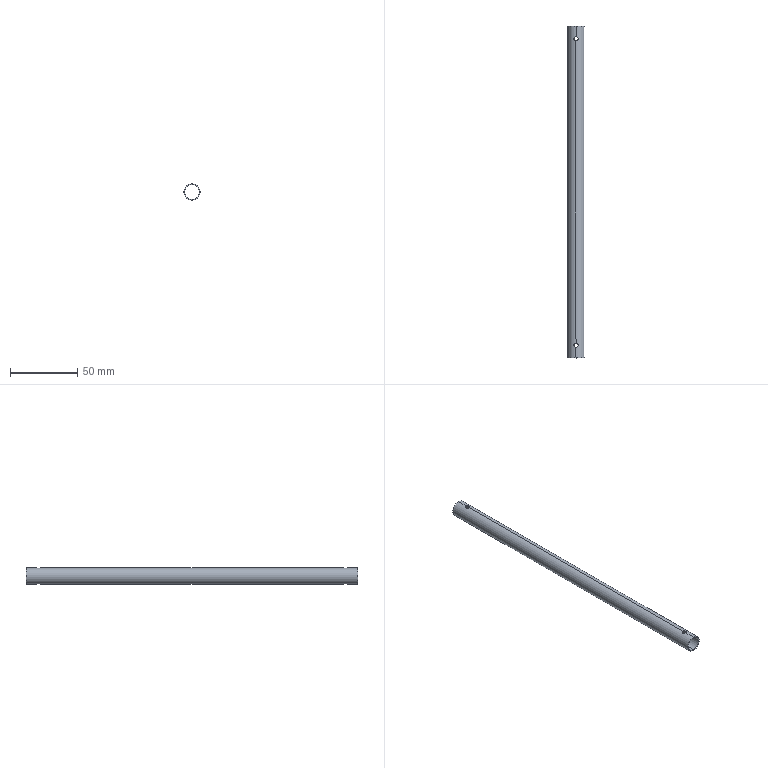Part | SolidWorks | features Extrusion 1, ICE 1 | 1 solid | 14 faces | box 12 x 246.5 x 12 mm | volume 4438 mm3 | cylinder 12 | plane 2 | commonest cylinder face diameters 3.1 x8 11 x2 12 x2
STEP:
#1=CARTESIAN_POINT('',(-1.55,237.,-5.796));
#2=VERTEX_POINT('',#1);
#3=CARTESIAN_POINT('',(0.,235.45,-6.));
#4=VERTEX_POINT('',#3);
#5=CARTESIAN_POINT('',(-1.55,237.,-5.796));
#6=CARTESIAN_POINT('',(-1.55,236.898,-5.796));
#7=CARTESIAN_POINT('',(-1.54,236.795,-5.799));
#8=CARTESIAN_POINT('',(-1.5,236.596,-5.81));
#9=CARTESIAN_POINT('',(-1.47,236.499,-5.817));
#10=CARTESIAN_POINT('',(-1.353,236.217,-5.846));
#11=CARTESIAN_POINT('',(-1.239,236.047,-5.872));
#12=CARTESIAN_POINT('',(-1.024,235.832,-5.912));
#13=CARTESIAN_POINT('',(-0.946,235.768,-5.926));
#14=CARTESIAN_POINT('',(-0.7784,235.656,-5.95));
#15=CARTESIAN_POINT('',(-0.6876,235.607,-5.961));
#16=CARTESIAN_POINT('',(-0.5006,235.53,-5.98));
#17=CARTESIAN_POINT('',(-0.404,235.5,-5.987));
#18=CARTESIAN_POINT('',(-0.2043,235.46,-5.997));
#19=CARTESIAN_POINT('',(-0.1014,235.45,-6.));
#20=CARTESIAN_POINT('',(0.,235.45,-6.));
#21=B_SPLINE_CURVE_WITH_KNOTS('',3,(#5,#6,#7,#8,#9,#10,#11,#12,#13,#14,#15,#16,#17,#18,#19,#20),.UNSPECIFIED.,.F.,.F.,(4,2,2,2,2,2,2,4),(0.002434,0.002738,0.003042,0.00365,0.003954,0.004259,0.004563,0.004867),.UNSPECIFIED.);
#22=EDGE_CURVE('',#2,#4,#21,.T.);
#23=ORIENTED_EDGE('',*,*,#22,.F.);
#24=CARTESIAN_POINT('',(-1.55,237.,-5.277));
#25=VERTEX_POINT('',#24);
#26=CARTESIAN_POINT('',(-1.55,237.,-6.));
#27=DIRECTION('',(0.,0.,1.));
#28=VECTOR('',#27,1000.);
#29=LINE('',#26,#28);
#30=EDGE_CURVE('',#2,#25,#29,.T.);
#31=ORIENTED_EDGE('',*,*,#30,.T.);
#32=CARTESIAN_POINT('',(0.,235.45,-5.5));
#33=VERTEX_POINT('',#32);
#34=CARTESIAN_POINT('',(-1.55,237.,-5.277));
#35=CARTESIAN_POINT('',(-1.55,236.898,-5.277));
#36=CARTESIAN_POINT('',(-1.54,236.795,-5.28));
#37=CARTESIAN_POINT('',(-1.5,236.596,-5.292));
#38=CARTESIAN_POINT('',(-1.47,236.499,-5.3));
#39=CARTESIAN_POINT('',(-1.353,236.217,-5.332));
#40=CARTESIAN_POINT('',(-1.239,236.047,-5.361));
#41=CARTESIAN_POINT('',(-1.024,235.832,-5.404));
#42=CARTESIAN_POINT('',(-0.9461,235.768,-5.419));
#43=CARTESIAN_POINT('',(-0.7786,235.656,-5.445));
#44=CARTESIAN_POINT('',(-0.6878,235.607,-5.458));
#45=CARTESIAN_POINT('',(-0.5009,235.53,-5.478));
#46=CARTESIAN_POINT('',(-0.4043,235.5,-5.486));
#47=CARTESIAN_POINT('',(-0.2043,235.46,-5.497));
#48=CARTESIAN_POINT('',(-0.1015,235.45,-5.5));
#49=CARTESIAN_POINT('',(0.,235.45,-5.5));
#50=B_SPLINE_CURVE_WITH_KNOTS('',3,(#34,#35,#36,#37,#38,#39,#40,#41,#42,#43,#44,#45,#46,#47,#48,#49),.UNSPECIFIED.,.F.,.F.,(4,2,2,2,2,2,2,4),(0.002436,0.00274,0.003045,0.003653,0.003958,0.004262,0.004566,0.004871),.UNSPECIFIED.);
#51=EDGE_CURVE('',#25,#33,#50,.T.);
#52=ORIENTED_EDGE('',*,*,#51,.T.);
#53=CARTESIAN_POINT('',(1.55,237.,-5.277));
#54=VERTEX_POINT('',#53);
#55=CARTESIAN_POINT('',(0.,235.45,-5.5));
#56=CARTESIAN_POINT('',(0.2029,235.45,-5.5));
#57=CARTESIAN_POINT('',(0.4079,235.491,-5.488));
#58=CARTESIAN_POINT('',(0.6881,235.607,-5.458));
#59=CARTESIAN_POINT('',(0.7788,235.656,-5.445));
#60=CARTESIAN_POINT('',(0.9467,235.769,-5.419));
#61=CARTESIAN_POINT('',(1.024,235.832,-5.404));
#62=CARTESIAN_POINT('',(1.167,235.975,-5.375));
#63=CARTESIAN_POINT('',(1.232,236.054,-5.36));
#64=CARTESIAN_POINT('',(1.344,236.222,-5.334));
#65=CARTESIAN_POINT('',(1.392,236.31,-5.321));
#66=CARTESIAN_POINT('',(1.47,236.499,-5.3));
#67=CARTESIAN_POINT('',(1.5,236.596,-5.292));
#68=CARTESIAN_POINT('',(1.54,236.795,-5.28));
#69=CARTESIAN_POINT('',(1.55,236.898,-5.277));
#70=CARTESIAN_POINT('',(1.55,237.,-5.277));
#71=B_SPLINE_CURVE_WITH_KNOTS('',3,(#55,#56,#57,#58,#59,#60,#61,#62,#63,#64,#65,#66,#67,#68,#69,#70),.UNSPECIFIED.,.F.,.F.,(4,2,2,2,2,2,2,4),(0.004871,0.00548,0.005784,0.006088,0.006393,0.006697,0.007001,0.007306),.UNSPECIFIED.);
#72=EDGE_CURVE('',#33,#54,#71,.T.);
#73=ORIENTED_EDGE('',*,*,#72,.T.);
#74=CARTESIAN_POINT('',(1.55,237.,-5.796));
#75=VERTEX_POINT('',#74);
#76=CARTESIAN_POINT('',(1.55,237.,-6.));
#77=DIRECTION('',(0.,0.,1.));
#78=VECTOR('',#77,1000.);
#79=LINE('',#76,#78);
#80=EDGE_CURVE('',#75,#54,#79,.T.);
#81=ORIENTED_EDGE('',*,*,#80,.F.);
#82=CARTESIAN_POINT('',(0.,235.45,-6.));
#83=CARTESIAN_POINT('',(0.2028,235.45,-6.));
#84=CARTESIAN_POINT('',(0.4076,235.491,-5.989));
#85=CARTESIAN_POINT('',(0.6877,235.607,-5.961));
#86=CARTESIAN_POINT('',(0.7784,235.656,-5.95));
#87=CARTESIAN_POINT('',(0.9465,235.768,-5.925));
#88=CARTESIAN_POINT('',(1.024,235.832,-5.912));
#89=CARTESIAN_POINT('',(1.167,235.975,-5.886));
#90=CARTESIAN_POINT('',(1.232,236.054,-5.872));
#91=CARTESIAN_POINT('',(1.344,236.222,-5.848));
#92=CARTESIAN_POINT('',(1.392,236.311,-5.836));
#93=CARTESIAN_POINT('',(1.51,236.594,-5.808));
#94=CARTESIAN_POINT('',(1.55,236.796,-5.796));
#95=CARTESIAN_POINT('',(1.55,237.,-5.796));
#96=B_SPLINE_CURVE_WITH_KNOTS('',3,(#82,#83,#84,#85,#86,#87,#88,#89,#90,#91,#92,#93,#94,#95),.UNSPECIFIED.,.F.,.F.,(4,2,2,2,2,2,4),(0.004867,0.005475,0.005779,0.006083,0.006387,0.006692,0.0073),.UNSPECIFIED.);
#97=EDGE_CURVE('',#4,#75,#96,.T.);
#98=ORIENTED_EDGE('',*,*,#97,.F.);
#99=EDGE_LOOP('',(#23,#31,#52,#73,#81,#98));
#100=FACE_OUTER_BOUND('',#99,.T.);
#101=CARTESIAN_POINT('',(0.,237.,-6.));
#102=DIRECTION('',(0.,0.,1.));
#103=DIRECTION('',(1.,0.,0.));
#104=AXIS2_PLACEMENT_3D('',#101,#102,#103);
#105=CYLINDRICAL_SURFACE('',#104,1.55);
#106=ADVANCED_FACE('',(#100),#105,.F.);
#107=CARTESIAN_POINT('',(0.,235.45,5.5));
#108=VERTEX_POINT('',#107);
#109=CARTESIAN_POINT('',(-1.55,237.,5.277));
#110=VERTEX_POINT('',#109);
#111=CARTESIAN_POINT('',(0.,235.45,5.5));
#112=CARTESIAN_POINT('',(-0.1017,235.45,5.5));
#113=CARTESIAN_POINT('',(-0.2049,235.46,5.497));
#114=CARTESIAN_POINT('',(-0.4041,235.5,5.486));
#115=CARTESIAN_POINT('',(-0.501,235.53,5.478));
#116=CARTESIAN_POINT('',(-0.7834,235.647,5.447));
#117=CARTESIAN_POINT('',(-0.9536,235.761,5.419));
#118=CARTESIAN_POINT('',(-1.168,235.976,5.375));
#119=CARTESIAN_POINT('',(-1.232,236.054,5.361));
#120=CARTESIAN_POINT('',(-1.344,236.222,5.334));
#121=CARTESIAN_POINT('',(-1.393,236.312,5.321));
#122=CARTESIAN_POINT('',(-1.47,236.499,5.3));
#123=CARTESIAN_POINT('',(-1.5,236.596,5.292));
#124=CARTESIAN_POINT('',(-1.54,236.796,5.28));
#125=CARTESIAN_POINT('',(-1.55,236.899,5.277));
#126=CARTESIAN_POINT('',(-1.55,237.,5.277));
#127=B_SPLINE_CURVE_WITH_KNOTS('',3,(#111,#112,#113,#114,#115,#116,#117,#118,#119,#120,#121,#122,#123,#124,#125,#126),.UNSPECIFIED.,.F.,.F.,(4,2,2,2,2,2,2,4),(0.002436,0.00274,0.003045,0.003653,0.003958,0.004262,0.004566,0.004871),.UNSPECIFIED.);
#128=EDGE_CURVE('',#108,#110,#127,.T.);
#129=ORIENTED_EDGE('',*,*,#128,.T.);
#130=CARTESIAN_POINT('',(-1.55,237.,5.796));
#131=VERTEX_POINT('',#130);
#132=CARTESIAN_POINT('',(-1.55,237.,-6.));
#133=DIRECTION('',(0.,0.,1.));
#134=VECTOR('',#133,1000.);
#135=LINE('',#132,#134);
#136=EDGE_CURVE('',#110,#131,#135,.T.);
#137=ORIENTED_EDGE('',*,*,#136,.T.);
#138=CARTESIAN_POINT('',(0.,235.45,6.));
#139=VERTEX_POINT('',#138);
#140=CARTESIAN_POINT('',(0.,235.45,6.));
#141=CARTESIAN_POINT('',(-0.1016,235.45,6.));
#142=CARTESIAN_POINT('',(-0.2048,235.46,5.997));
#143=CARTESIAN_POINT('',(-0.4038,235.5,5.987));
#144=CARTESIAN_POINT('',(-0.5007,235.53,5.98));
#145=CARTESIAN_POINT('',(-0.7829,235.647,5.952));
#146=CARTESIAN_POINT('',(-0.9532,235.761,5.926));
#147=CARTESIAN_POINT('',(-1.168,235.976,5.886));
#148=CARTESIAN_POINT('',(-1.232,236.054,5.872));
#149=CARTESIAN_POINT('',(-1.344,236.222,5.848));
#150=CARTESIAN_POINT('',(-1.393,236.312,5.836));
#151=CARTESIAN_POINT('',(-1.47,236.499,5.817));
#152=CARTESIAN_POINT('',(-1.5,236.596,5.81));
#153=CARTESIAN_POINT('',(-1.54,236.796,5.799));
#154=CARTESIAN_POINT('',(-1.55,236.899,5.796));
#155=CARTESIAN_POINT('',(-1.55,237.,5.796));
#156=B_SPLINE_CURVE_WITH_KNOTS('',3,(#140,#141,#142,#143,#144,#145,#146,#147,#148,#149,#150,#151,#152,#153,#154,#155),.UNSPECIFIED.,.F.,.F.,(4,2,2,2,2,2,2,4),(0.002434,0.002738,0.003042,0.00365,0.003954,0.004259,0.004563,0.004867),.UNSPECIFIED.);
#157=EDGE_CURVE('',#139,#131,#156,.T.);
#158=ORIENTED_EDGE('',*,*,#157,.F.);
#159=CARTESIAN_POINT('',(1.55,237.,5.796));
#160=VERTEX_POINT('',#159);
#161=CARTESIAN_POINT('',(1.55,237.,5.796));
#162=CARTESIAN_POINT('',(1.55,236.897,5.796));
#163=CARTESIAN_POINT('',(1.54,236.796,5.799));
#164=CARTESIAN_POINT('',(1.5,236.597,5.809));
#165=CARTESIAN_POINT('',(1.47,236.499,5.817));
#166=CARTESIAN_POINT('',(1.392,236.311,5.836));
#167=CARTESIAN_POINT('',(1.344,236.222,5.848));
#168=CARTESIAN_POINT('',(1.232,236.054,5.872));
#169=CARTESIAN_POINT('',(1.167,235.975,5.886));
#170=CARTESIAN_POINT('',(0.9531,235.761,5.926));
#171=CARTESIAN_POINT('',(0.7808,235.646,5.952));
#172=CARTESIAN_POINT('',(0.4079,235.491,5.989));
#173=CARTESIAN_POINT('',(0.2032,235.45,6.));
#174=CARTESIAN_POINT('',(0.,235.45,6.));
#175=B_SPLINE_CURVE_WITH_KNOTS('',3,(#161,#162,#163,#164,#165,#166,#167,#168,#169,#170,#171,#172,#173,#174),.UNSPECIFIED.,.F.,.F.,(4,2,2,2,2,2,4),(0.,0.0003042,0.0006085,0.0009127,0.001217,0.001825,0.002434),.UNSPECIFIED.);
#176=EDGE_CURVE('',#160,#139,#175,.T.);
#177=ORIENTED_EDGE('',*,*,#176,.F.);
#178=CARTESIAN_POINT('',(1.55,237.,5.277));
#179=VERTEX_POINT('',#178);
#180=CARTESIAN_POINT('',(1.55,237.,-6.));
#181=DIRECTION('',(0.,0.,1.));
#182=VECTOR('',#181,1000.);
#183=LINE('',#180,#182);
#184=EDGE_CURVE('',#179,#160,#183,.T.);
#185=ORIENTED_EDGE('',*,*,#184,.F.);
#186=CARTESIAN_POINT('',(1.55,237.,5.277));
#187=CARTESIAN_POINT('',(1.55,236.897,5.277));
#188=CARTESIAN_POINT('',(1.54,236.796,5.28));
#189=CARTESIAN_POINT('',(1.5,236.597,5.292));
#190=CARTESIAN_POINT('',(1.47,236.498,5.3));
#191=CARTESIAN_POINT('',(1.392,236.311,5.321));
#192=CARTESIAN_POINT('',(1.344,236.222,5.333));
#193=CARTESIAN_POINT('',(1.232,236.054,5.361));
#194=CARTESIAN_POINT('',(1.167,235.975,5.375));
#195=CARTESIAN_POINT('',(0.9533,235.761,5.419));
#196=CARTESIAN_POINT('',(0.7811,235.646,5.447));
#197=CARTESIAN_POINT('',(0.4082,235.491,5.488));
#198=CARTESIAN_POINT('',(0.2034,235.45,5.5));
#199=CARTESIAN_POINT('',(0.,235.45,5.5));
#200=B_SPLINE_CURVE_WITH_KNOTS('',3,(#186,#187,#188,#189,#190,#191,#192,#193,#194,#195,#196,#197,#198,#199),.UNSPECIFIED.,.F.,.F.,(4,2,2,2,2,2,4),(0.,0.0003045,0.000609,0.0009135,0.001218,0.001827,0.002436),.UNSPECIFIED.);
#201=EDGE_CURVE('',#179,#108,#200,.T.);
#202=ORIENTED_EDGE('',*,*,#201,.T.);
#203=EDGE_LOOP('',(#129,#137,#158,#177,#185,#202));
#204=FACE_OUTER_BOUND('',#203,.T.);
#205=CARTESIAN_POINT('',(0.,237.,-6.));
#206=DIRECTION('',(0.,0.,1.));
#207=DIRECTION('',(1.,0.,0.));
#208=AXIS2_PLACEMENT_3D('',#205,#206,#207);
#209=CYLINDRICAL_SURFACE('',#208,1.55);
#210=ADVANCED_FACE('',(#204),#209,.F.);
#211=CARTESIAN_POINT('',(-1.55,9.5,-5.796));
#212=VERTEX_POINT('',#211);
#213=CARTESIAN_POINT('',(0.,7.95,-6.));
#214=VERTEX_POINT('',#213);
#215=CARTESIAN_POINT('',(-1.55,9.5,-5.796));
#216=CARTESIAN_POINT('',(-1.55,9.398,-5.796));
#217=CARTESIAN_POINT('',(-1.54,9.295,-5.799));
#218=CARTESIAN_POINT('',(-1.5,9.096,-5.81));
#219=CARTESIAN_POINT('',(-1.47,8.999,-5.817));
#220=CARTESIAN_POINT('',(-1.353,8.717,-5.846));
#221=CARTESIAN_POINT('',(-1.239,8.547,-5.872));
#222=CARTESIAN_POINT('',(-1.024,8.332,-5.912));
#223=CARTESIAN_POINT('',(-0.946,8.268,-5.926));
#224=CARTESIAN_POINT('',(-0.7784,8.156,-5.95));
#225=CARTESIAN_POINT('',(-0.6876,8.107,-5.961));
#226=CARTESIAN_POINT('',(-0.5006,8.03,-5.98));
#227=CARTESIAN_POINT('',(-0.404,8.,-5.987));
#228=CARTESIAN_POINT('',(-0.2043,7.96,-5.997));
#229=CARTESIAN_POINT('',(-0.1014,7.95,-6.));
#230=CARTESIAN_POINT('',(0.,7.95,-6.));
#231=B_SPLINE_CURVE_WITH_KNOTS('',3,(#215,#216,#217,#218,#219,#220,#221,#222,#223,#224,#225,#226,#227,#228,#229,#230),.UNSPECIFIED.,.F.,.F.,(4,2,2,2,2,2,2,4),(0.002434,0.002738,0.003042,0.00365,0.003954,0.004259,0.004563,0.004867),.UNSPECIFIED.);
#232=EDGE_CURVE('',#212,#214,#231,.T.);
#233=ORIENTED_EDGE('',*,*,#232,.F.);
#234=CARTESIAN_POINT('',(-1.55,9.5,-5.277));
#235=VERTEX_POINT('',#234);
#236=CARTESIAN_POINT('',(-1.55,9.5,-6.));
#237=DIRECTION('',(0.,0.,1.));
#238=VECTOR('',#237,1000.);
#239=LINE('',#236,#238);
#240=EDGE_CURVE('',#212,#235,#239,.T.);
#241=ORIENTED_EDGE('',*,*,#240,.T.);
#242=CARTESIAN_POINT('',(0.,7.95,-5.5));
#243=VERTEX_POINT('',#242);
#244=CARTESIAN_POINT('',(-1.55,9.5,-5.277));
#245=CARTESIAN_POINT('',(-1.55,9.398,-5.277));
#246=CARTESIAN_POINT('',(-1.54,9.295,-5.28));
#247=CARTESIAN_POINT('',(-1.5,9.096,-5.292));
#248=CARTESIAN_POINT('',(-1.47,8.999,-5.3));
#249=CARTESIAN_POINT('',(-1.353,8.717,-5.332));
#250=CARTESIAN_POINT('',(-1.239,8.547,-5.361));
#251=CARTESIAN_POINT('',(-1.024,8.332,-5.404));
#252=CARTESIAN_POINT('',(-0.9461,8.268,-5.419));
#253=CARTESIAN_POINT('',(-0.7786,8.156,-5.445));
#254=CARTESIAN_POINT('',(-0.6878,8.107,-5.458));
#255=CARTESIAN_POINT('',(-0.5009,8.03,-5.478));
#256=CARTESIAN_POINT('',(-0.4043,8.,-5.486));
#257=CARTESIAN_POINT('',(-0.2043,7.96,-5.497));
#258=CARTESIAN_POINT('',(-0.1015,7.95,-5.5));
#259=CARTESIAN_POINT('',(0.,7.95,-5.5));
#260=B_SPLINE_CURVE_WITH_KNOTS('',3,(#244,#245,#246,#247,#248,#249,#250,#251,#252,#253,#254,#255,#256,#257,#258,#259),.UNSPECIFIED.,.F.,.F.,(4,2,2,2,2,2,2,4),(0.002436,0.00274,0.003045,0.003653,0.003958,0.004262,0.004566,0.004871),.UNSPECIFIED.);
#261=EDGE_CURVE('',#235,#243,#260,.T.);
#262=ORIENTED_EDGE('',*,*,#261,.T.);
#263=CARTESIAN_POINT('',(1.55,9.5,-5.277));
#264=VERTEX_POINT('',#263);
#265=CARTESIAN_POINT('',(0.,7.95,-5.5));
#266=CARTESIAN_POINT('',(0.2029,7.95,-5.5));
#267=CARTESIAN_POINT('',(0.4079,7.991,-5.488));
#268=CARTESIAN_POINT('',(0.6881,8.107,-5.458));
#269=CARTESIAN_POINT('',(0.7788,8.156,-5.445));
#270=CARTESIAN_POINT('',(0.9467,8.269,-5.419));
#271=CARTESIAN_POINT('',(1.024,8.332,-5.404));
#272=CARTESIAN_POINT('',(1.167,8.475,-5.375));
#273=CARTESIAN_POINT('',(1.232,8.554,-5.36));
#274=CARTESIAN_POINT('',(1.344,8.722,-5.334));
#275=CARTESIAN_POINT('',(1.392,8.81,-5.321));
#276=CARTESIAN_POINT('',(1.47,8.999,-5.3));
#277=CARTESIAN_POINT('',(1.5,9.096,-5.292));
#278=CARTESIAN_POINT('',(1.54,9.295,-5.28));
#279=CARTESIAN_POINT('',(1.55,9.398,-5.277));
#280=CARTESIAN_POINT('',(1.55,9.5,-5.277));
#281=B_SPLINE_CURVE_WITH_KNOTS('',3,(#265,#266,#267,#268,#269,#270,#271,#272,#273,#274,#275,#276,#277,#278,#279,#280),.UNSPECIFIED.,.F.,.F.,(4,2,2,2,2,2,2,4),(0.004871,0.00548,0.005784,0.006088,0.006393,0.006697,0.007001,0.007306),.UNSPECIFIED.);
#282=EDGE_CURVE('',#243,#264,#281,.T.);
#283=ORIENTED_EDGE('',*,*,#282,.T.);
#284=CARTESIAN_POINT('',(1.55,9.5,-5.796));
#285=VERTEX_POINT('',#284);
#286=CARTESIAN_POINT('',(1.55,9.5,-6.));
#287=DIRECTION('',(0.,0.,1.));
#288=VECTOR('',#287,1000.);
#289=LINE('',#286,#288);
#290=EDGE_CURVE('',#285,#264,#289,.T.);
#291=ORIENTED_EDGE('',*,*,#290,.F.);
#292=CARTESIAN_POINT('',(0.,7.95,-6.));
#293=CARTESIAN_POINT('',(0.2028,7.95,-6.));
#294=CARTESIAN_POINT('',(0.4076,7.991,-5.989));
#295=CARTESIAN_POINT('',(0.6877,8.107,-5.961));
#296=CARTESIAN_POINT('',(0.7784,8.156,-5.95));
#297=CARTESIAN_POINT('',(0.9465,8.268,-5.925));
#298=CARTESIAN_POINT('',(1.024,8.332,-5.912));
#299=CARTESIAN_POINT('',(1.167,8.475,-5.886));
#300=CARTESIAN_POINT('',(1.232,8.554,-5.872));
#301=CARTESIAN_POINT('',(1.344,8.722,-5.848));
#302=CARTESIAN_POINT('',(1.392,8.811,-5.836));
#303=CARTESIAN_POINT('',(1.51,9.094,-5.808));
#304=CARTESIAN_POINT('',(1.55,9.296,-5.796));
#305=CARTESIAN_POINT('',(1.55,9.5,-5.796));
#306=B_SPLINE_CURVE_WITH_KNOTS('',3,(#292,#293,#294,#295,#296,#297,#298,#299,#300,#301,#302,#303,#304,#305),.UNSPECIFIED.,.F.,.F.,(4,2,2,2,2,2,4),(0.004867,0.005475,0.005779,0.006083,0.006387,0.006692,0.0073),.UNSPECIFIED.);
#307=EDGE_CURVE('',#214,#285,#306,.T.);
#308=ORIENTED_EDGE('',*,*,#307,.F.);
#309=EDGE_LOOP('',(#233,#241,#262,#283,#291,#308));
#310=FACE_OUTER_BOUND('',#309,.T.);
#311=CARTESIAN_POINT('',(0.,9.5,-6.));
#312=DIRECTION('',(0.,0.,1.));
#313=DIRECTION('',(1.,0.,0.));
#314=AXIS2_PLACEMENT_3D('',#311,#312,#313);
#315=CYLINDRICAL_SURFACE('',#314,1.55);
#316=ADVANCED_FACE('',(#310),#315,.F.);
#317=CARTESIAN_POINT('',(0.,7.95,5.5));
#318=VERTEX_POINT('',#317);
#319=CARTESIAN_POINT('',(-1.55,9.5,5.277));
#320=VERTEX_POINT('',#319);
#321=CARTESIAN_POINT('',(0.,7.95,5.5));
#322=CARTESIAN_POINT('',(-0.1017,7.95,5.5));
#323=CARTESIAN_POINT('',(-0.2049,7.96,5.497));
#324=CARTESIAN_POINT('',(-0.4041,8.,5.486));
#325=CARTESIAN_POINT('',(-0.501,8.03,5.478));
#326=CARTESIAN_POINT('',(-0.7834,8.147,5.447));
#327=CARTESIAN_POINT('',(-0.9536,8.261,5.419));
#328=CARTESIAN_POINT('',(-1.168,8.476,5.375));
#329=CARTESIAN_POINT('',(-1.232,8.554,5.361));
#330=CARTESIAN_POINT('',(-1.344,8.722,5.334));
#331=CARTESIAN_POINT('',(-1.393,8.812,5.321));
#332=CARTESIAN_POINT('',(-1.47,8.999,5.3));
#333=CARTESIAN_POINT('',(-1.5,9.096,5.292));
#334=CARTESIAN_POINT('',(-1.54,9.296,5.28));
#335=CARTESIAN_POINT('',(-1.55,9.399,5.277));
#336=CARTESIAN_POINT('',(-1.55,9.5,5.277));
#337=B_SPLINE_CURVE_WITH_KNOTS('',3,(#321,#322,#323,#324,#325,#326,#327,#328,#329,#330,#331,#332,#333,#334,#335,#336),.UNSPECIFIED.,.F.,.F.,(4,2,2,2,2,2,2,4),(0.002436,0.00274,0.003045,0.003653,0.003958,0.004262,0.004566,0.004871),.UNSPECIFIED.);
#338=EDGE_CURVE('',#318,#320,#337,.T.);
#339=ORIENTED_EDGE('',*,*,#338,.T.);
#340=CARTESIAN_POINT('',(-1.55,9.5,5.796));
#341=VERTEX_POINT('',#340);
#342=CARTESIAN_POINT('',(-1.55,9.5,-6.));
#343=DIRECTION('',(0.,0.,1.));
#344=VECTOR('',#343,1000.);
#345=LINE('',#342,#344);
#346=EDGE_CURVE('',#320,#341,#345,.T.);
#347=ORIENTED_EDGE('',*,*,#346,.T.);
#348=CARTESIAN_POINT('',(0.,7.95,6.));
#349=VERTEX_POINT('',#348);
#350=CARTESIAN_POINT('',(0.,7.95,6.));
#351=CARTESIAN_POINT('',(-0.1016,7.95,6.));
#352=CARTESIAN_POINT('',(-0.2048,7.96,5.997));
#353=CARTESIAN_POINT('',(-0.4038,8.,5.987));
#354=CARTESIAN_POINT('',(-0.5007,8.03,5.98));
#355=CARTESIAN_POINT('',(-0.7829,8.147,5.952));
#356=CARTESIAN_POINT('',(-0.9532,8.261,5.926));
#357=CARTESIAN_POINT('',(-1.168,8.476,5.886));
#358=CARTESIAN_POINT('',(-1.232,8.554,5.872));
#359=CARTESIAN_POINT('',(-1.344,8.722,5.848));
#360=CARTESIAN_POINT('',(-1.393,8.812,5.836));
#361=CARTESIAN_POINT('',(-1.47,8.999,5.817));
#362=CARTESIAN_POINT('',(-1.5,9.096,5.81));
#363=CARTESIAN_POINT('',(-1.54,9.296,5.799));
#364=CARTESIAN_POINT('',(-1.55,9.399,5.796));
#365=CARTESIAN_POINT('',(-1.55,9.5,5.796));
#366=B_SPLINE_CURVE_WITH_KNOTS('',3,(#350,#351,#352,#353,#354,#355,#356,#357,#358,#359,#360,#361,#362,#363,#364,#365),.UNSPECIFIED.,.F.,.F.,(4,2,2,2,2,2,2,4),(0.002434,0.002738,0.003042,0.00365,0.003954,0.004259,0.004563,0.004867),.UNSPECIFIED.);
#367=EDGE_CURVE('',#349,#341,#366,.T.);
#368=ORIENTED_EDGE('',*,*,#367,.F.);
#369=CARTESIAN_POINT('',(1.55,9.5,5.796));
#370=VERTEX_POINT('',#369);
#371=CARTESIAN_POINT('',(1.55,9.5,5.796));
#372=CARTESIAN_POINT('',(1.55,9.397,5.796));
#373=CARTESIAN_POINT('',(1.54,9.296,5.799));
#374=CARTESIAN_POINT('',(1.5,9.097,5.809));
#375=CARTESIAN_POINT('',(1.47,8.999,5.817));
#376=CARTESIAN_POINT('',(1.392,8.811,5.836));
#377=CARTESIAN_POINT('',(1.344,8.722,5.848));
#378=CARTESIAN_POINT('',(1.232,8.554,5.872));
#379=CARTESIAN_POINT('',(1.167,8.475,5.886));
#380=CARTESIAN_POINT('',(0.9531,8.261,5.926));
#381=CARTESIAN_POINT('',(0.7808,8.146,5.952));
#382=CARTESIAN_POINT('',(0.4079,7.991,5.989));
#383=CARTESIAN_POINT('',(0.2032,7.95,6.));
#384=CARTESIAN_POINT('',(0.,7.95,6.));
#385=B_SPLINE_CURVE_WITH_KNOTS('',3,(#371,#372,#373,#374,#375,#376,#377,#378,#379,#380,#381,#382,#383,#384),.UNSPECIFIED.,.F.,.F.,(4,2,2,2,2,2,4),(0.,0.0003042,0.0006085,0.0009127,0.001217,0.001825,0.002434),.UNSPECIFIED.);
#386=EDGE_CURVE('',#370,#349,#385,.T.);
#387=ORIENTED_EDGE('',*,*,#386,.F.);
#388=CARTESIAN_POINT('',(1.55,9.5,5.277));
#389=VERTEX_POINT('',#388);
#390=CARTESIAN_POINT('',(1.55,9.5,-6.));
#391=DIRECTION('',(0.,0.,1.));
#392=VECTOR('',#391,1000.);
#393=LINE('',#390,#392);
#394=EDGE_CURVE('',#389,#370,#393,.T.);
#395=ORIENTED_EDGE('',*,*,#394,.F.);
#396=CARTESIAN_POINT('',(1.55,9.5,5.277));
#397=CARTESIAN_POINT('',(1.55,9.397,5.277));
#398=CARTESIAN_POINT('',(1.54,9.296,5.28));
#399=CARTESIAN_POINT('',(1.5,9.097,5.292));
#400=CARTESIAN_POINT('',(1.47,8.998,5.3));
#401=CARTESIAN_POINT('',(1.392,8.811,5.321));
#402=CARTESIAN_POINT('',(1.344,8.722,5.333));
#403=CARTESIAN_POINT('',(1.232,8.554,5.361));
#404=CARTESIAN_POINT('',(1.167,8.475,5.375));
#405=CARTESIAN_POINT('',(0.9533,8.261,5.419));
#406=CARTESIAN_POINT('',(0.7811,8.146,5.447));
#407=CARTESIAN_POINT('',(0.4082,7.991,5.488));
#408=CARTESIAN_POINT('',(0.2034,7.95,5.5));
#409=CARTESIAN_POINT('',(0.,7.95,5.5));
#410=B_SPLINE_CURVE_WITH_KNOTS('',3,(#396,#397,#398,#399,#400,#401,#402,#403,#404,#405,#406,#407,#408,#409),.UNSPECIFIED.,.F.,.F.,(4,2,2,2,2,2,4),(0.,0.0003045,0.000609,0.0009135,0.001218,0.001827,0.002436),.UNSPECIFIED.);
#411=EDGE_CURVE('',#389,#318,#410,.T.);
#412=ORIENTED_EDGE('',*,*,#411,.T.);
#413=EDGE_LOOP('',(#339,#347,#368,#387,#395,#412));
#414=FACE_OUTER_BOUND('',#413,.T.);
#415=CARTESIAN_POINT('',(0.,9.5,-6.));
#416=DIRECTION('',(0.,0.,1.));
#417=DIRECTION('',(1.,0.,0.));
#418=AXIS2_PLACEMENT_3D('',#415,#416,#417);
#419=CYLINDRICAL_SURFACE('',#418,1.55);
#420=ADVANCED_FACE('',(#414),#419,.F.);
#421=CARTESIAN_POINT('',(0.,246.5,-5.5));
#422=VERTEX_POINT('',#421);
#423=CARTESIAN_POINT('',(0.,246.5,5.5));
#424=VERTEX_POINT('',#423);
#425=CARTESIAN_POINT('',(0.,246.5,0.));
#426=DIRECTION('',(0.,1.,0.));
#427=DIRECTION('',(0.,0.,1.));
#428=AXIS2_PLACEMENT_3D('',#425,#426,#427);
#429=CIRCLE('',#428,5.5);
#430=EDGE_CURVE('',#422,#424,#429,.T.);
#431=ORIENTED_EDGE('',*,*,#430,.T.);
#432=CARTESIAN_POINT('',(0.,238.55,5.5));
#433=VERTEX_POINT('',#432);
#434=CARTESIAN_POINT('',(0.,246.5,5.5));
#435=DIRECTION('',(0.,-1.,0.));
#436=VECTOR('',#435,1000.);
#437=LINE('',#434,#436);
#438=EDGE_CURVE('',#424,#433,#437,.T.);
#439=ORIENTED_EDGE('',*,*,#438,.T.);
#440=CARTESIAN_POINT('',(-1.55,237.,5.277));
#441=CARTESIAN_POINT('',(-1.55,237.203,5.277));
#442=CARTESIAN_POINT('',(-1.509,237.408,5.29));
#443=CARTESIAN_POINT('',(-1.393,237.688,5.321));
#444=CARTESIAN_POINT('',(-1.344,237.779,5.334));
#445=CARTESIAN_POINT('',(-1.232,237.946,5.361));
#446=CARTESIAN_POINT('',(-1.168,238.024,5.375));
#447=CARTESIAN_POINT('',(-1.025,238.167,5.404));
#448=CARTESIAN_POINT('',(-0.9458,238.232,5.419));
#449=CARTESIAN_POINT('',(-0.7786,238.344,5.445));
#450=CARTESIAN_POINT('',(-0.6897,238.392,5.457));
#451=CARTESIAN_POINT('',(-0.5007,238.47,5.478));
#452=CARTESIAN_POINT('',(-0.4036,238.5,5.486));
#453=CARTESIAN_POINT('',(-0.205,238.54,5.497));
#454=CARTESIAN_POINT('',(-0.1022,238.55,5.5));
#455=CARTESIAN_POINT('',(0.,238.55,5.5));
#456=B_SPLINE_CURVE_WITH_KNOTS('',3,(#440,#441,#442,#443,#444,#445,#446,#447,#448,#449,#450,#451,#452,#453,#454,#455),.UNSPECIFIED.,.F.,.F.,(4,2,2,2,2,2,2,4),(0.004871,0.005479,0.005784,0.006088,0.006393,0.006697,0.007001,0.007306),.UNSPECIFIED.);
#457=EDGE_CURVE('',#110,#433,#456,.T.);
#458=ORIENTED_EDGE('',*,*,#457,.F.);
#459=ORIENTED_EDGE('',*,*,#128,.F.);
#460=CARTESIAN_POINT('',(0.,11.05,5.5));
#461=VERTEX_POINT('',#460);
#462=CARTESIAN_POINT('',(0.,246.5,5.5));
#463=DIRECTION('',(0.,-1.,0.));
#464=VECTOR('',#463,1000.);
#465=LINE('',#462,#464);
#466=EDGE_CURVE('',#108,#461,#465,.T.);
#467=ORIENTED_EDGE('',*,*,#466,.T.);
#468=CARTESIAN_POINT('',(-1.55,9.5,5.277));
#469=CARTESIAN_POINT('',(-1.55,9.703,5.277));
#470=CARTESIAN_POINT('',(-1.509,9.908,5.29));
#471=CARTESIAN_POINT('',(-1.393,10.188,5.321));
#472=CARTESIAN_POINT('',(-1.344,10.279,5.334));
#473=CARTESIAN_POINT('',(-1.232,10.446,5.361));
#474=CARTESIAN_POINT('',(-1.168,10.524,5.375));
#475=CARTESIAN_POINT('',(-1.025,10.667,5.404));
#476=CARTESIAN_POINT('',(-0.9458,10.732,5.419));
#477=CARTESIAN_POINT('',(-0.7786,10.844,5.445));
#478=CARTESIAN_POINT('',(-0.6897,10.892,5.457));
#479=CARTESIAN_POINT('',(-0.5007,10.97,5.478));
#480=CARTESIAN_POINT('',(-0.4036,11.,5.486));
#481=CARTESIAN_POINT('',(-0.205,11.04,5.497));
#482=CARTESIAN_POINT('',(-0.1022,11.05,5.5));
#483=CARTESIAN_POINT('',(0.,11.05,5.5));
#484=B_SPLINE_CURVE_WITH_KNOTS('',3,(#468,#469,#470,#471,#472,#473,#474,#475,#476,#477,#478,#479,#480,#481,#482,#483),.UNSPECIFIED.,.F.,.F.,(4,2,2,2,2,2,2,4),(0.004871,0.005479,0.005784,0.006088,0.006393,0.006697,0.007001,0.007306),.UNSPECIFIED.);
#485=EDGE_CURVE('',#320,#461,#484,.T.);
#486=ORIENTED_EDGE('',*,*,#485,.F.);
#487=ORIENTED_EDGE('',*,*,#338,.F.);
#488=CARTESIAN_POINT('',(0.,0.,5.5));
#489=VERTEX_POINT('',#488);
#490=CARTESIAN_POINT('',(0.,246.5,5.5));
#491=DIRECTION('',(0.,-1.,0.));
#492=VECTOR('',#491,1000.);
#493=LINE('',#490,#492);
#494=EDGE_CURVE('',#318,#489,#493,.T.);
#495=ORIENTED_EDGE('',*,*,#494,.T.);
#496=CARTESIAN_POINT('',(0.,0.,-5.5));
#497=VERTEX_POINT('',#496);
#498=CARTESIAN_POINT('',(0.,0.,0.));
#499=DIRECTION('',(0.,1.,0.));
#500=DIRECTION('',(0.,0.,1.));
#501=AXIS2_PLACEMENT_3D('',#498,#499,#500);
#502=CIRCLE('',#501,5.5);
#503=EDGE_CURVE('',#497,#489,#502,.T.);
#504=ORIENTED_EDGE('',*,*,#503,.F.);
#505=CARTESIAN_POINT('',(0.,246.5,-5.5));
#506=DIRECTION('',(0.,-1.,0.));
#507=VECTOR('',#506,1000.);
#508=LINE('',#505,#507);
#509=EDGE_CURVE('',#243,#497,#508,.T.);
#510=ORIENTED_EDGE('',*,*,#509,.F.);
#511=ORIENTED_EDGE('',*,*,#261,.F.);
#512=CARTESIAN_POINT('',(0.,11.05,-5.5));
#513=VERTEX_POINT('',#512);
#514=CARTESIAN_POINT('',(0.,11.05,-5.5));
#515=CARTESIAN_POINT('',(-0.103,11.05,-5.5));
#516=CARTESIAN_POINT('',(-0.2042,11.04,-5.497));
#517=CARTESIAN_POINT('',(-0.4031,11.,-5.486));
#518=CARTESIAN_POINT('',(-0.5018,10.97,-5.478));
#519=CARTESIAN_POINT('',(-0.6894,10.892,-5.457));
#520=CARTESIAN_POINT('',(-0.7782,10.844,-5.445));
#521=CARTESIAN_POINT('',(-0.9464,10.732,-5.419));
#522=CARTESIAN_POINT('',(-1.026,10.667,-5.404));
#523=CARTESIAN_POINT('',(-1.239,10.453,-5.361));
#524=CARTESIAN_POINT('',(-1.354,10.281,-5.331));
#525=CARTESIAN_POINT('',(-1.509,9.908,-5.29));
#526=CARTESIAN_POINT('',(-1.55,9.703,-5.277));
#527=CARTESIAN_POINT('',(-1.55,9.5,-5.277));
#528=B_SPLINE_CURVE_WITH_KNOTS('',3,(#514,#515,#516,#517,#518,#519,#520,#521,#522,#523,#524,#525,#526,#527),.UNSPECIFIED.,.F.,.F.,(4,2,2,2,2,2,4),(0.,0.0003045,0.000609,0.0009135,0.001218,0.001827,0.002436),.UNSPECIFIED.);
#529=EDGE_CURVE('',#513,#235,#528,.T.);
#530=ORIENTED_EDGE('',*,*,#529,.F.);
#531=CARTESIAN_POINT('',(0.,246.5,-5.5));
#532=DIRECTION('',(0.,-1.,0.));
#533=VECTOR('',#532,1000.);
#534=LINE('',#531,#533);
#535=EDGE_CURVE('',#33,#513,#534,.T.);
#536=ORIENTED_EDGE('',*,*,#535,.F.);
#537=ORIENTED_EDGE('',*,*,#51,.F.);
#538=CARTESIAN_POINT('',(0.,238.55,-5.5));
#539=VERTEX_POINT('',#538);
#540=CARTESIAN_POINT('',(0.,238.55,-5.5));
#541=CARTESIAN_POINT('',(-0.103,238.55,-5.5));
#542=CARTESIAN_POINT('',(-0.2042,238.54,-5.497));
#543=CARTESIAN_POINT('',(-0.4031,238.5,-5.486));
#544=CARTESIAN_POINT('',(-0.5018,238.47,-5.478));
#545=CARTESIAN_POINT('',(-0.6894,238.392,-5.457));
#546=CARTESIAN_POINT('',(-0.7782,238.344,-5.445));
#547=CARTESIAN_POINT('',(-0.9464,238.232,-5.419));
#548=CARTESIAN_POINT('',(-1.026,238.167,-5.404));
#549=CARTESIAN_POINT('',(-1.239,237.953,-5.361));
#550=CARTESIAN_POINT('',(-1.354,237.781,-5.331));
#551=CARTESIAN_POINT('',(-1.509,237.408,-5.29));
#552=CARTESIAN_POINT('',(-1.55,237.203,-5.277));
#553=CARTESIAN_POINT('',(-1.55,237.,-5.277));
#554=B_SPLINE_CURVE_WITH_KNOTS('',3,(#540,#541,#542,#543,#544,#545,#546,#547,#548,#549,#550,#551,#552,#553),.UNSPECIFIED.,.F.,.F.,(4,2,2,2,2,2,4),(0.,0.0003045,0.000609,0.0009135,0.001218,0.001827,0.002436),.UNSPECIFIED.);
#555=EDGE_CURVE('',#539,#25,#554,.T.);
#556=ORIENTED_EDGE('',*,*,#555,.F.);
#557=CARTESIAN_POINT('',(0.,246.5,-5.5));
#558=DIRECTION('',(0.,-1.,0.));
#559=VECTOR('',#558,1000.);
#560=LINE('',#557,#559);
#561=EDGE_CURVE('',#422,#539,#560,.T.);
#562=ORIENTED_EDGE('',*,*,#561,.F.);
#563=EDGE_LOOP('',(#431,#439,#458,#459,#467,#486,#487,#495,#504,#510,#511,#530,#536,#537,#556,#562));
#564=FACE_OUTER_BOUND('',#563,.T.);
#565=CARTESIAN_POINT('',(0.,246.5,0.));
#566=DIRECTION('',(0.,-1.,0.));
#567=DIRECTION('',(0.,0.,-1.));
#568=AXIS2_PLACEMENT_3D('',#565,#566,#567);
#569=CYLINDRICAL_SURFACE('',#568,5.5);
#570=ADVANCED_FACE('',(#564),#569,.F.);
#571=CARTESIAN_POINT('',(0.,246.5,6.));
#572=VERTEX_POINT('',#571);
#573=CARTESIAN_POINT('',(0.,246.5,-6.));
#574=VERTEX_POINT('',#573);
#575=CARTESIAN_POINT('',(0.,246.5,0.));
#576=DIRECTION('',(0.,1.,0.));
#577=DIRECTION('',(0.,0.,1.));
#578=AXIS2_PLACEMENT_3D('',#575,#576,#577);
#579=CIRCLE('',#578,6.);
#580=EDGE_CURVE('',#572,#574,#579,.T.);
#581=ORIENTED_EDGE('',*,*,#580,.F.);
#582=CARTESIAN_POINT('',(0.,238.55,6.));
#583=VERTEX_POINT('',#582);
#584=CARTESIAN_POINT('',(0.,246.5,6.));
#585=DIRECTION('',(0.,-1.,0.));
#586=VECTOR('',#585,1000.);
#587=LINE('',#584,#586);
#588=EDGE_CURVE('',#572,#583,#587,.T.);
#589=ORIENTED_EDGE('',*,*,#588,.T.);
#590=CARTESIAN_POINT('',(0.,238.55,6.));
#591=CARTESIAN_POINT('',(0.1022,238.55,6.));
#592=CARTESIAN_POINT('',(0.2031,238.54,5.997));
#593=CARTESIAN_POINT('',(0.4022,238.5,5.987));
#594=CARTESIAN_POINT('',(0.5011,238.47,5.98));
#595=CARTESIAN_POINT('',(0.7814,238.354,5.952));
#596=CARTESIAN_POINT('',(0.9534,238.239,5.926));
#597=CARTESIAN_POINT('',(1.238,237.954,5.873));
#598=CARTESIAN_POINT('',(1.353,237.782,5.846));
#599=CARTESIAN_POINT('',(1.47,237.503,5.817));
#600=CARTESIAN_POINT('',(1.5,237.404,5.81));
#601=CARTESIAN_POINT('',(1.54,237.204,5.799));
#602=CARTESIAN_POINT('',(1.55,237.103,5.796));
#603=CARTESIAN_POINT('',(1.55,237.,5.796));
#604=B_SPLINE_CURVE_WITH_KNOTS('',3,(#590,#591,#592,#593,#594,#595,#596,#597,#598,#599,#600,#601,#602,#603),.UNSPECIFIED.,.F.,.F.,(4,2,2,2,2,2,4),(0.0073,0.007604,0.007908,0.008516,0.009124,0.009428,0.009732),.UNSPECIFIED.);
#605=EDGE_CURVE('',#583,#160,#604,.T.);
#606=ORIENTED_EDGE('',*,*,#605,.T.);
#607=ORIENTED_EDGE('',*,*,#176,.T.);
#608=CARTESIAN_POINT('',(0.,11.05,6.));
#609=VERTEX_POINT('',#608);
#610=CARTESIAN_POINT('',(0.,246.5,6.));
#611=DIRECTION('',(0.,-1.,0.));
#612=VECTOR('',#611,1000.);
#613=LINE('',#610,#612);
#614=EDGE_CURVE('',#139,#609,#613,.T.);
#615=ORIENTED_EDGE('',*,*,#614,.T.);
#616=CARTESIAN_POINT('',(0.,11.05,6.));
#617=CARTESIAN_POINT('',(0.1022,11.05,6.));
#618=CARTESIAN_POINT('',(0.2031,11.04,5.997));
#619=CARTESIAN_POINT('',(0.4022,11.,5.987));
#620=CARTESIAN_POINT('',(0.5011,10.97,5.98));
#621=CARTESIAN_POINT('',(0.7814,10.854,5.952));
#622=CARTESIAN_POINT('',(0.9534,10.739,5.926));
#623=CARTESIAN_POINT('',(1.238,10.454,5.873));
#624=CARTESIAN_POINT('',(1.353,10.282,5.846));
#625=CARTESIAN_POINT('',(1.47,10.003,5.817));
#626=CARTESIAN_POINT('',(1.5,9.904,5.81));
#627=CARTESIAN_POINT('',(1.54,9.704,5.799));
#628=CARTESIAN_POINT('',(1.55,9.603,5.796));
#629=CARTESIAN_POINT('',(1.55,9.5,5.796));
#630=B_SPLINE_CURVE_WITH_KNOTS('',3,(#616,#617,#618,#619,#620,#621,#622,#623,#624,#625,#626,#627,#628,#629),.UNSPECIFIED.,.F.,.F.,(4,2,2,2,2,2,4),(0.0073,0.007604,0.007908,0.008516,0.009124,0.009428,0.009732),.UNSPECIFIED.);
#631=EDGE_CURVE('',#609,#370,#630,.T.);
#632=ORIENTED_EDGE('',*,*,#631,.T.);
#633=ORIENTED_EDGE('',*,*,#386,.T.);
#634=CARTESIAN_POINT('',(0.,0.,6.));
#635=VERTEX_POINT('',#634);
#636=CARTESIAN_POINT('',(0.,246.5,6.));
#637=DIRECTION('',(0.,-1.,0.));
#638=VECTOR('',#637,1000.);
#639=LINE('',#636,#638);
#640=EDGE_CURVE('',#349,#635,#639,.T.);
#641=ORIENTED_EDGE('',*,*,#640,.T.);
#642=CARTESIAN_POINT('',(0.,0.,-6.));
#643=VERTEX_POINT('',#642);
#644=CARTESIAN_POINT('',(0.,0.,0.));
#645=DIRECTION('',(0.,1.,0.));
#646=DIRECTION('',(0.,0.,1.));
#647=AXIS2_PLACEMENT_3D('',#644,#645,#646);
#648=CIRCLE('',#647,6.);
#649=EDGE_CURVE('',#635,#643,#648,.T.);
#650=ORIENTED_EDGE('',*,*,#649,.T.);
#651=CARTESIAN_POINT('',(0.,246.5,-6.));
#652=DIRECTION('',(0.,-1.,0.));
#653=VECTOR('',#652,1000.);
#654=LINE('',#651,#653);
#655=EDGE_CURVE('',#214,#643,#654,.T.);
#656=ORIENTED_EDGE('',*,*,#655,.F.);
#657=ORIENTED_EDGE('',*,*,#307,.T.);
#658=CARTESIAN_POINT('',(0.,11.05,-6.));
#659=VERTEX_POINT('',#658);
#660=CARTESIAN_POINT('',(1.55,9.5,-5.796));
#661=CARTESIAN_POINT('',(1.55,9.602,-5.796));
#662=CARTESIAN_POINT('',(1.54,9.703,-5.799));
#663=CARTESIAN_POINT('',(1.5,9.902,-5.809));
#664=CARTESIAN_POINT('',(1.47,10.001,-5.817));
#665=CARTESIAN_POINT('',(1.354,10.281,-5.846));
#666=CARTESIAN_POINT('',(1.239,10.453,-5.873));
#667=CARTESIAN_POINT('',(0.9543,10.738,-5.925));
#668=CARTESIAN_POINT('',(0.7825,10.853,-5.952));
#669=CARTESIAN_POINT('',(0.5026,10.97,-5.98));
#670=CARTESIAN_POINT('',(0.4038,11.,-5.987));
#671=CARTESIAN_POINT('',(0.2042,11.04,-5.997));
#672=CARTESIAN_POINT('',(0.1028,11.05,-6.));
#673=CARTESIAN_POINT('',(0.,11.05,-6.));
#674=B_SPLINE_CURVE_WITH_KNOTS('',3,(#660,#661,#662,#663,#664,#665,#666,#667,#668,#669,#670,#671,#672,#673),.UNSPECIFIED.,.F.,.F.,(4,2,2,2,2,2,4),(0.0073,0.007604,0.007908,0.008516,0.009124,0.009428,0.009732),.UNSPECIFIED.);
#675=EDGE_CURVE('',#285,#659,#674,.T.);
#676=ORIENTED_EDGE('',*,*,#675,.T.);
#677=CARTESIAN_POINT('',(0.,246.5,-6.));
#678=DIRECTION('',(0.,-1.,0.));
#679=VECTOR('',#678,1000.);
#680=LINE('',#677,#679);
#681=EDGE_CURVE('',#4,#659,#680,.T.);
#682=ORIENTED_EDGE('',*,*,#681,.F.);
#683=ORIENTED_EDGE('',*,*,#97,.T.);
#684=CARTESIAN_POINT('',(0.,238.55,-6.));
#685=VERTEX_POINT('',#684);
#686=CARTESIAN_POINT('',(1.55,237.,-5.796));
#687=CARTESIAN_POINT('',(1.55,237.102,-5.796));
#688=CARTESIAN_POINT('',(1.54,237.203,-5.799));
#689=CARTESIAN_POINT('',(1.5,237.402,-5.809));
#690=CARTESIAN_POINT('',(1.47,237.501,-5.817));
#691=CARTESIAN_POINT('',(1.354,237.781,-5.846));
#692=CARTESIAN_POINT('',(1.239,237.953,-5.873));
#693=CARTESIAN_POINT('',(0.9543,238.238,-5.925));
#694=CARTESIAN_POINT('',(0.7825,238.353,-5.952));
#695=CARTESIAN_POINT('',(0.5026,238.47,-5.98));
#696=CARTESIAN_POINT('',(0.4038,238.5,-5.987));
#697=CARTESIAN_POINT('',(0.2042,238.54,-5.997));
#698=CARTESIAN_POINT('',(0.1028,238.55,-6.));
#699=CARTESIAN_POINT('',(0.,238.55,-6.));
#700=B_SPLINE_CURVE_WITH_KNOTS('',3,(#686,#687,#688,#689,#690,#691,#692,#693,#694,#695,#696,#697,#698,#699),.UNSPECIFIED.,.F.,.F.,(4,2,2,2,2,2,4),(0.0073,0.007604,0.007908,0.008516,0.009124,0.009428,0.009732),.UNSPECIFIED.);
#701=EDGE_CURVE('',#75,#685,#700,.T.);
#702=ORIENTED_EDGE('',*,*,#701,.T.);
#703=CARTESIAN_POINT('',(0.,246.5,-6.));
#704=DIRECTION('',(0.,-1.,0.));
#705=VECTOR('',#704,1000.);
#706=LINE('',#703,#705);
#707=EDGE_CURVE('',#574,#685,#706,.T.);
#708=ORIENTED_EDGE('',*,*,#707,.F.);
#709=EDGE_LOOP('',(#581,#589,#606,#607,#615,#632,#633,#641,#650,#656,#657,#676,#682,#683,#702,#708));
#710=FACE_OUTER_BOUND('',#709,.T.);
#711=CARTESIAN_POINT('',(0.,246.5,0.));
#712=DIRECTION('',(0.,-1.,0.));
#713=DIRECTION('',(0.,0.,-1.));
#714=AXIS2_PLACEMENT_3D('',#711,#712,#713);
#715=CYLINDRICAL_SURFACE('',#714,6.);
#716=ADVANCED_FACE('',(#710),#715,.T.);
#717=CARTESIAN_POINT('',(0.,246.5,0.));
#718=DIRECTION('',(0.,1.,0.));
#719=DIRECTION('',(0.,0.,1.));
#720=AXIS2_PLACEMENT_3D('',#717,#718,#719);
#721=CIRCLE('',#720,6.);
#722=EDGE_CURVE('',#574,#572,#721,.T.);
#723=ORIENTED_EDGE('',*,*,#722,.T.);
#724=ORIENTED_EDGE('',*,*,#580,.T.);
#725=EDGE_LOOP('',(#723,#724));
#726=FACE_OUTER_BOUND('',#725,.T.);
#727=ORIENTED_EDGE('',*,*,#430,.F.);
#728=CARTESIAN_POINT('',(0.,246.5,0.));
#729=DIRECTION('',(0.,1.,0.));
#730=DIRECTION('',(0.,0.,1.));
#731=AXIS2_PLACEMENT_3D('',#728,#729,#730);
#732=CIRCLE('',#731,5.5);
#733=EDGE_CURVE('',#424,#422,#732,.T.);
#734=ORIENTED_EDGE('',*,*,#733,.F.);
#735=EDGE_LOOP('',(#727,#734));
#736=FACE_BOUND('',#735,.T.);
#737=CARTESIAN_POINT('',(0.,246.5,0.));
#738=DIRECTION('',(0.,1.,0.));
#739=DIRECTION('',(0.,0.,1.));
#740=AXIS2_PLACEMENT_3D('',#737,#738,#739);
#741=PLANE('',#740);
#742=ADVANCED_FACE('',(#726,#736),#741,.T.);
#743=CARTESIAN_POINT('',(0.,0.,0.));
#744=DIRECTION('',(0.,1.,0.));
#745=DIRECTION('',(0.,0.,1.));
#746=AXIS2_PLACEMENT_3D('',#743,#744,#745);
#747=CIRCLE('',#746,6.);
#748=EDGE_CURVE('',#643,#635,#747,.T.);
#749=ORIENTED_EDGE('',*,*,#748,.F.);
#750=ORIENTED_EDGE('',*,*,#649,.F.);
#751=EDGE_LOOP('',(#749,#750));
#752=FACE_OUTER_BOUND('',#751,.T.);
#753=ORIENTED_EDGE('',*,*,#503,.T.);
#754=CARTESIAN_POINT('',(0.,0.,0.));
#755=DIRECTION('',(0.,1.,0.));
#756=DIRECTION('',(0.,0.,1.));
#757=AXIS2_PLACEMENT_3D('',#754,#755,#756);
#758=CIRCLE('',#757,5.5);
#759=EDGE_CURVE('',#489,#497,#758,.T.);
#760=ORIENTED_EDGE('',*,*,#759,.T.);
#761=EDGE_LOOP('',(#753,#760));
#762=FACE_BOUND('',#761,.T.);
#763=CARTESIAN_POINT('',(0.,0.,0.));
#764=DIRECTION('',(0.,1.,0.));
#765=DIRECTION('',(0.,0.,1.));
#766=AXIS2_PLACEMENT_3D('',#763,#764,#765);
#767=PLANE('',#766);
#768=ADVANCED_FACE('',(#752,#762),#767,.F.);
#769=ORIENTED_EDGE('',*,*,#588,.F.);
#770=ORIENTED_EDGE('',*,*,#722,.F.);
#771=ORIENTED_EDGE('',*,*,#707,.T.);
#772=CARTESIAN_POINT('',(0.,238.55,-6.));
#773=CARTESIAN_POINT('',(-0.1029,238.55,-6.));
#774=CARTESIAN_POINT('',(-0.204,238.54,-5.997));
#775=CARTESIAN_POINT('',(-0.4028,238.5,-5.987));
#776=CARTESIAN_POINT('',(-0.5015,238.47,-5.98));
#777=CARTESIAN_POINT('',(-0.6891,238.392,-5.961));
#778=CARTESIAN_POINT('',(-0.778,238.344,-5.95));
#779=CARTESIAN_POINT('',(-0.9462,238.232,-5.926));
#780=CARTESIAN_POINT('',(-1.025,238.167,-5.912));
#781=CARTESIAN_POINT('',(-1.239,237.953,-5.872));
#782=CARTESIAN_POINT('',(-1.354,237.781,-5.846));
#783=CARTESIAN_POINT('',(-1.509,237.408,-5.808));
#784=CARTESIAN_POINT('',(-1.55,237.203,-5.796));
#785=CARTESIAN_POINT('',(-1.55,237.,-5.796));
#786=B_SPLINE_CURVE_WITH_KNOTS('',3,(#772,#773,#774,#775,#776,#777,#778,#779,#780,#781,#782,#783,#784,#785),.UNSPECIFIED.,.F.,.F.,(4,2,2,2,2,2,4),(0.,0.0003043,0.0006085,0.0009128,0.001217,0.001826,0.002434),.UNSPECIFIED.);
#787=EDGE_CURVE('',#685,#2,#786,.T.);
#788=ORIENTED_EDGE('',*,*,#787,.T.);
#789=ORIENTED_EDGE('',*,*,#22,.T.);
#790=ORIENTED_EDGE('',*,*,#681,.T.);
#791=CARTESIAN_POINT('',(0.,11.05,-6.));
#792=CARTESIAN_POINT('',(-0.1029,11.05,-6.));
#793=CARTESIAN_POINT('',(-0.204,11.04,-5.997));
#794=CARTESIAN_POINT('',(-0.4028,11.,-5.987));
#795=CARTESIAN_POINT('',(-0.5015,10.97,-5.98));
#796=CARTESIAN_POINT('',(-0.6891,10.892,-5.961));
#797=CARTESIAN_POINT('',(-0.778,10.844,-5.95));
#798=CARTESIAN_POINT('',(-0.9462,10.732,-5.926));
#799=CARTESIAN_POINT('',(-1.025,10.667,-5.912));
#800=CARTESIAN_POINT('',(-1.239,10.453,-5.872));
#801=CARTESIAN_POINT('',(-1.354,10.281,-5.846));
#802=CARTESIAN_POINT('',(-1.509,9.908,-5.808));
#803=CARTESIAN_POINT('',(-1.55,9.703,-5.796));
#804=CARTESIAN_POINT('',(-1.55,9.5,-5.796));
#805=B_SPLINE_CURVE_WITH_KNOTS('',3,(#791,#792,#793,#794,#795,#796,#797,#798,#799,#800,#801,#802,#803,#804),.UNSPECIFIED.,.F.,.F.,(4,2,2,2,2,2,4),(0.,0.0003043,0.0006085,0.0009128,0.001217,0.001826,0.002434),.UNSPECIFIED.);
#806=EDGE_CURVE('',#659,#212,#805,.T.);
#807=ORIENTED_EDGE('',*,*,#806,.T.);
#808=ORIENTED_EDGE('',*,*,#232,.T.);
#809=ORIENTED_EDGE('',*,*,#655,.T.);
#810=ORIENTED_EDGE('',*,*,#748,.T.);
#811=ORIENTED_EDGE('',*,*,#640,.F.);
#812=ORIENTED_EDGE('',*,*,#367,.T.);
#813=CARTESIAN_POINT('',(-1.55,9.5,5.796));
#814=CARTESIAN_POINT('',(-1.55,9.703,5.796));
#815=CARTESIAN_POINT('',(-1.509,9.908,5.808));
#816=CARTESIAN_POINT('',(-1.393,10.188,5.836));
#817=CARTESIAN_POINT('',(-1.344,10.278,5.848));
#818=CARTESIAN_POINT('',(-1.232,10.446,5.873));
#819=CARTESIAN_POINT('',(-1.168,10.524,5.886));
#820=CARTESIAN_POINT('',(-1.025,10.667,5.912));
#821=CARTESIAN_POINT('',(-0.9457,10.732,5.926));
#822=CARTESIAN_POINT('',(-0.7783,10.844,5.95));
#823=CARTESIAN_POINT('',(-0.6894,10.892,5.961));
#824=CARTESIAN_POINT('',(-0.4063,11.01,5.989));
#825=CARTESIAN_POINT('',(-0.2045,11.05,6.));
#826=CARTESIAN_POINT('',(0.,11.05,6.));
#827=B_SPLINE_CURVE_WITH_KNOTS('',3,(#813,#814,#815,#816,#817,#818,#819,#820,#821,#822,#823,#824,#825,#826),.UNSPECIFIED.,.F.,.F.,(4,2,2,2,2,2,4),(0.004867,0.005475,0.005779,0.006083,0.006387,0.006691,0.0073),.UNSPECIFIED.);
#828=EDGE_CURVE('',#341,#609,#827,.T.);
#829=ORIENTED_EDGE('',*,*,#828,.T.);
#830=ORIENTED_EDGE('',*,*,#614,.F.);
#831=ORIENTED_EDGE('',*,*,#157,.T.);
#832=CARTESIAN_POINT('',(-1.55,237.,5.796));
#833=CARTESIAN_POINT('',(-1.55,237.203,5.796));
#834=CARTESIAN_POINT('',(-1.509,237.408,5.808));
#835=CARTESIAN_POINT('',(-1.393,237.688,5.836));
#836=CARTESIAN_POINT('',(-1.344,237.778,5.848));
#837=CARTESIAN_POINT('',(-1.232,237.946,5.873));
#838=CARTESIAN_POINT('',(-1.168,238.024,5.886));
#839=CARTESIAN_POINT('',(-1.025,238.167,5.912));
#840=CARTESIAN_POINT('',(-0.9457,238.232,5.926));
#841=CARTESIAN_POINT('',(-0.7783,238.344,5.95));
#842=CARTESIAN_POINT('',(-0.6894,238.392,5.961));
#843=CARTESIAN_POINT('',(-0.4063,238.51,5.989));
#844=CARTESIAN_POINT('',(-0.2045,238.55,6.));
#845=CARTESIAN_POINT('',(0.,238.55,6.));
#846=B_SPLINE_CURVE_WITH_KNOTS('',3,(#832,#833,#834,#835,#836,#837,#838,#839,#840,#841,#842,#843,#844,#845),.UNSPECIFIED.,.F.,.F.,(4,2,2,2,2,2,4),(0.004867,0.005475,0.005779,0.006083,0.006387,0.006691,0.0073),.UNSPECIFIED.);
#847=EDGE_CURVE('',#131,#583,#846,.T.);
#848=ORIENTED_EDGE('',*,*,#847,.T.);
#849=EDGE_LOOP('',(#769,#770,#771,#788,#789,#790,#807,#808,#809,#810,#811,#812,#829,#830,#831,#848));
#850=FACE_OUTER_BOUND('',#849,.T.);
#851=CARTESIAN_POINT('',(0.,246.5,0.));
#852=DIRECTION('',(0.,-1.,0.));
#853=DIRECTION('',(0.,0.,-1.));
#854=AXIS2_PLACEMENT_3D('',#851,#852,#853);
#855=CYLINDRICAL_SURFACE('',#854,6.);
#856=ADVANCED_FACE('',(#850),#855,.T.);
#857=ORIENTED_EDGE('',*,*,#438,.F.);
#858=ORIENTED_EDGE('',*,*,#733,.T.);
#859=ORIENTED_EDGE('',*,*,#561,.T.);
#860=CARTESIAN_POINT('',(1.55,237.,-5.277));
#861=CARTESIAN_POINT('',(1.55,237.102,-5.277));
#862=CARTESIAN_POINT('',(1.54,237.203,-5.28));
#863=CARTESIAN_POINT('',(1.5,237.403,-5.291));
#864=CARTESIAN_POINT('',(1.47,237.501,-5.3));
#865=CARTESIAN_POINT('',(1.354,237.782,-5.331));
#866=CARTESIAN_POINT('',(1.239,237.953,-5.361));
#867=CARTESIAN_POINT('',(0.9544,238.238,-5.419));
#868=CARTESIAN_POINT('',(0.7828,238.353,-5.447));
#869=CARTESIAN_POINT('',(0.5027,238.47,-5.478));
#870=CARTESIAN_POINT('',(0.4038,238.5,-5.486));
#871=CARTESIAN_POINT('',(0.2043,238.54,-5.497));
#872=CARTESIAN_POINT('',(0.1029,238.55,-5.5));
#873=CARTESIAN_POINT('',(0.,238.55,-5.5));
#874=B_SPLINE_CURVE_WITH_KNOTS('',3,(#860,#861,#862,#863,#864,#865,#866,#867,#868,#869,#870,#871,#872,#873),.UNSPECIFIED.,.F.,.F.,(4,2,2,2,2,2,4),(0.007306,0.00761,0.007914,0.008523,0.009132,0.009436,0.00974),.UNSPECIFIED.);
#875=EDGE_CURVE('',#54,#539,#874,.T.);
#876=ORIENTED_EDGE('',*,*,#875,.F.);
#877=ORIENTED_EDGE('',*,*,#72,.F.);
#878=ORIENTED_EDGE('',*,*,#535,.T.);
#879=CARTESIAN_POINT('',(1.55,9.5,-5.277));
#880=CARTESIAN_POINT('',(1.55,9.602,-5.277));
#881=CARTESIAN_POINT('',(1.54,9.703,-5.28));
#882=CARTESIAN_POINT('',(1.5,9.903,-5.291));
#883=CARTESIAN_POINT('',(1.47,10.001,-5.3));
#884=CARTESIAN_POINT('',(1.354,10.282,-5.331));
#885=CARTESIAN_POINT('',(1.239,10.453,-5.361));
#886=CARTESIAN_POINT('',(0.9544,10.738,-5.419));
#887=CARTESIAN_POINT('',(0.7828,10.853,-5.447));
#888=CARTESIAN_POINT('',(0.5027,10.97,-5.478));
#889=CARTESIAN_POINT('',(0.4038,11.,-5.486));
#890=CARTESIAN_POINT('',(0.2043,11.04,-5.497));
#891=CARTESIAN_POINT('',(0.1029,11.05,-5.5));
#892=CARTESIAN_POINT('',(0.,11.05,-5.5));
#893=B_SPLINE_CURVE_WITH_KNOTS('',3,(#879,#880,#881,#882,#883,#884,#885,#886,#887,#888,#889,#890,#891,#892),.UNSPECIFIED.,.F.,.F.,(4,2,2,2,2,2,4),(0.007306,0.00761,0.007914,0.008523,0.009132,0.009436,0.00974),.UNSPECIFIED.);
#894=EDGE_CURVE('',#264,#513,#893,.T.);
#895=ORIENTED_EDGE('',*,*,#894,.F.);
#896=ORIENTED_EDGE('',*,*,#282,.F.);
#897=ORIENTED_EDGE('',*,*,#509,.T.);
#898=ORIENTED_EDGE('',*,*,#759,.F.);
#899=ORIENTED_EDGE('',*,*,#494,.F.);
#900=ORIENTED_EDGE('',*,*,#411,.F.);
#901=CARTESIAN_POINT('',(0.,11.05,5.5));
#902=CARTESIAN_POINT('',(0.1022,11.05,5.5));
#903=CARTESIAN_POINT('',(0.2031,11.04,5.497));
#904=CARTESIAN_POINT('',(0.4026,11.,5.486));
#905=CARTESIAN_POINT('',(0.5015,10.97,5.478));
#906=CARTESIAN_POINT('',(0.7817,10.854,5.447));
#907=CARTESIAN_POINT('',(0.9536,10.738,5.419));
#908=CARTESIAN_POINT('',(1.238,10.454,5.361));
#909=CARTESIAN_POINT('',(1.353,10.283,5.332));
#910=CARTESIAN_POINT('',(1.47,10.003,5.3));
#911=CARTESIAN_POINT('',(1.5,9.904,5.292));
#912=CARTESIAN_POINT('',(1.54,9.704,5.28));
#913=CARTESIAN_POINT('',(1.55,9.603,5.277));
#914=CARTESIAN_POINT('',(1.55,9.5,5.277));
#915=B_SPLINE_CURVE_WITH_KNOTS('',3,(#901,#902,#903,#904,#905,#906,#907,#908,#909,#910,#911,#912,#913,#914),.UNSPECIFIED.,.F.,.F.,(4,2,2,2,2,2,4),(0.007306,0.00761,0.007914,0.008523,0.009132,0.009436,0.00974),.UNSPECIFIED.);
#916=EDGE_CURVE('',#461,#389,#915,.T.);
#917=ORIENTED_EDGE('',*,*,#916,.F.);
#918=ORIENTED_EDGE('',*,*,#466,.F.);
#919=ORIENTED_EDGE('',*,*,#201,.F.);
#920=CARTESIAN_POINT('',(0.,238.55,5.5));
#921=CARTESIAN_POINT('',(0.1022,238.55,5.5));
#922=CARTESIAN_POINT('',(0.2031,238.54,5.497));
#923=CARTESIAN_POINT('',(0.4026,238.5,5.486));
#924=CARTESIAN_POINT('',(0.5015,238.47,5.478));
#925=CARTESIAN_POINT('',(0.7817,238.354,5.447));
#926=CARTESIAN_POINT('',(0.9536,238.238,5.419));
#927=CARTESIAN_POINT('',(1.238,237.954,5.361));
#928=CARTESIAN_POINT('',(1.353,237.783,5.332));
#929=CARTESIAN_POINT('',(1.47,237.503,5.3));
#930=CARTESIAN_POINT('',(1.5,237.404,5.292));
#931=CARTESIAN_POINT('',(1.54,237.204,5.28));
#932=CARTESIAN_POINT('',(1.55,237.103,5.277));
#933=CARTESIAN_POINT('',(1.55,237.,5.277));
#934=B_SPLINE_CURVE_WITH_KNOTS('',3,(#920,#921,#922,#923,#924,#925,#926,#927,#928,#929,#930,#931,#932,#933),.UNSPECIFIED.,.F.,.F.,(4,2,2,2,2,2,4),(0.007306,0.00761,0.007914,0.008523,0.009132,0.009436,0.00974),.UNSPECIFIED.);
#935=EDGE_CURVE('',#433,#179,#934,.T.);
#936=ORIENTED_EDGE('',*,*,#935,.F.);
#937=EDGE_LOOP('',(#857,#858,#859,#876,#877,#878,#895,#896,#897,#898,#899,#900,#917,#918,#919,#936));
#938=FACE_OUTER_BOUND('',#937,.T.);
#939=CARTESIAN_POINT('',(0.,246.5,0.));
#940=DIRECTION('',(0.,-1.,0.));
#941=DIRECTION('',(0.,0.,-1.));
#942=AXIS2_PLACEMENT_3D('',#939,#940,#941);
#943=CYLINDRICAL_SURFACE('',#942,5.5);
#944=ADVANCED_FACE('',(#938),#943,.F.);
#945=ORIENTED_EDGE('',*,*,#346,.F.);
#946=ORIENTED_EDGE('',*,*,#485,.T.);
#947=ORIENTED_EDGE('',*,*,#916,.T.);
#948=ORIENTED_EDGE('',*,*,#394,.T.);
#949=ORIENTED_EDGE('',*,*,#631,.F.);
#950=ORIENTED_EDGE('',*,*,#828,.F.);
#951=EDGE_LOOP('',(#945,#946,#947,#948,#949,#950));
#952=FACE_OUTER_BOUND('',#951,.T.);
#953=CARTESIAN_POINT('',(0.,9.5,-6.));
#954=DIRECTION('',(0.,0.,1.));
#955=DIRECTION('',(1.,0.,0.));
#956=AXIS2_PLACEMENT_3D('',#953,#954,#955);
#957=CYLINDRICAL_SURFACE('',#956,1.55);
#958=ADVANCED_FACE('',(#952),#957,.F.);
#959=ORIENTED_EDGE('',*,*,#240,.F.);
#960=ORIENTED_EDGE('',*,*,#806,.F.);
#961=ORIENTED_EDGE('',*,*,#675,.F.);
#962=ORIENTED_EDGE('',*,*,#290,.T.);
#963=ORIENTED_EDGE('',*,*,#894,.T.);
#964=ORIENTED_EDGE('',*,*,#529,.T.);
#965=EDGE_LOOP('',(#959,#960,#961,#962,#963,#964));
#966=FACE_OUTER_BOUND('',#965,.T.);
#967=CARTESIAN_POINT('',(0.,9.5,-6.));
#968=DIRECTION('',(0.,0.,1.));
#969=DIRECTION('',(1.,0.,0.));
#970=AXIS2_PLACEMENT_3D('',#967,#968,#969);
#971=CYLINDRICAL_SURFACE('',#970,1.55);
#972=ADVANCED_FACE('',(#966),#971,.F.);
#973=ORIENTED_EDGE('',*,*,#136,.F.);
#974=ORIENTED_EDGE('',*,*,#457,.T.);
#975=ORIENTED_EDGE('',*,*,#935,.T.);
#976=ORIENTED_EDGE('',*,*,#184,.T.);
#977=ORIENTED_EDGE('',*,*,#605,.F.);
#978=ORIENTED_EDGE('',*,*,#847,.F.);
#979=EDGE_LOOP('',(#973,#974,#975,#976,#977,#978));
#980=FACE_OUTER_BOUND('',#979,.T.);
#981=CARTESIAN_POINT('',(0.,237.,-6.));
#982=DIRECTION('',(0.,0.,1.));
#983=DIRECTION('',(1.,0.,0.));
#984=AXIS2_PLACEMENT_3D('',#981,#982,#983);
#985=CYLINDRICAL_SURFACE('',#984,1.55);
#986=ADVANCED_FACE('',(#980),#985,.F.);
#987=ORIENTED_EDGE('',*,*,#30,.F.);
#988=ORIENTED_EDGE('',*,*,#787,.F.);
#989=ORIENTED_EDGE('',*,*,#701,.F.);
#990=ORIENTED_EDGE('',*,*,#80,.T.);
#991=ORIENTED_EDGE('',*,*,#875,.T.);
#992=ORIENTED_EDGE('',*,*,#555,.T.);
#993=EDGE_LOOP('',(#987,#988,#989,#990,#991,#992));
#994=FACE_OUTER_BOUND('',#993,.T.);
#995=CARTESIAN_POINT('',(0.,237.,-6.));
#996=DIRECTION('',(0.,0.,1.));
#997=DIRECTION('',(1.,0.,0.));
#998=AXIS2_PLACEMENT_3D('',#995,#996,#997);
#999=CYLINDRICAL_SURFACE('',#998,1.55);
#1000=ADVANCED_FACE('',(#994),#999,.F.);
#1001=CLOSED_SHELL('',(#106,#210,#316,#420,#570,#716,#742,#768,#856,#944,#958,#972,#986,#1000));
#1002=MANIFOLD_SOLID_BREP('',#1001);
#1003=CARTESIAN_POINT('',(0.,0.,0.));
#1004=DIRECTION('',(0.,0.,1.));
#1005=DIRECTION('',(1.,0.,0.));
#1006=AXIS2_PLACEMENT_3D('',#1003,#1004,#1005);
#1007=(LENGTH_UNIT()NAMED_UNIT(*)SI_UNIT(.MILLI.,.METRE.));
#1008=UNCERTAINTY_MEASURE_WITH_UNIT(LENGTH_MEASURE(0.00001),#1007,'','');
#1009=(NAMED_UNIT(*)PLANE_ANGLE_UNIT()SI_UNIT($,.RADIAN.));
#1010=(NAMED_UNIT(*)SI_UNIT($,.STERADIAN.)SOLID_ANGLE_UNIT());
#1011=(GEOMETRIC_REPRESENTATION_CONTEXT(3)GLOBAL_UNCERTAINTY_ASSIGNED_CONTEXT((#1008))GLOBAL_UNIT_ASSIGNED_CONTEXT((#1007,#1009,#1010))REPRESENTATION_CONTEXT('',''));
#1012=ADVANCED_BREP_SHAPE_REPRESENTATION('',(#1002,#1006),#1011);